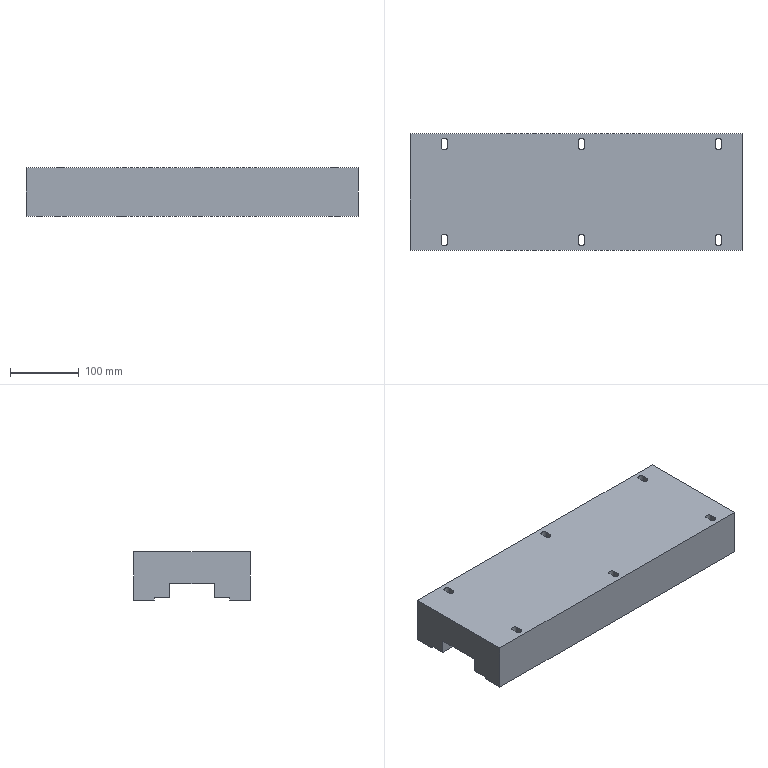Part | STEP file | PN_0007 Fixing plate | 1 solid | 220 faces | box 484 x 170 x 70 mm | volume 4861056 mm3 | cylinder 100 | cone 76 | plane 44 | commonest cylinder face diameters 2.5 x68 9 x12 15 x12 6.8 x8